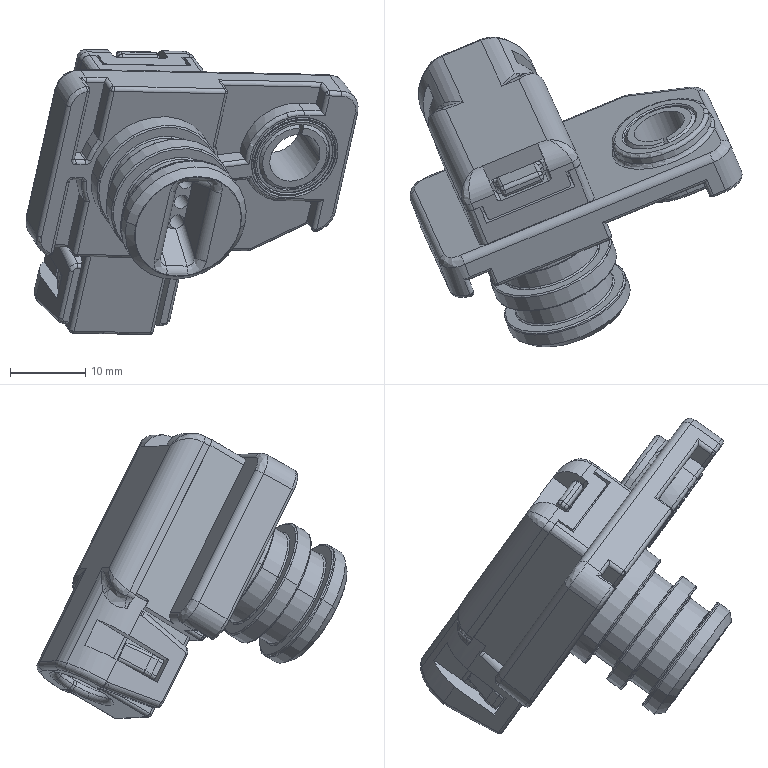Part | SolidWorks | features BaseBody 1 | 1 solid | 770 faces | box 44.308 x 41.304 x 38.03 mm | volume 10705 mm3 | cylinder 267 | plane 194 | spline 135 | torus 76 | cone 51 | sphere 47 | commonest cylinder face diameters 1 x124 2 x53 6 x14 17.05 x8 11.26 x6 13.6 x6